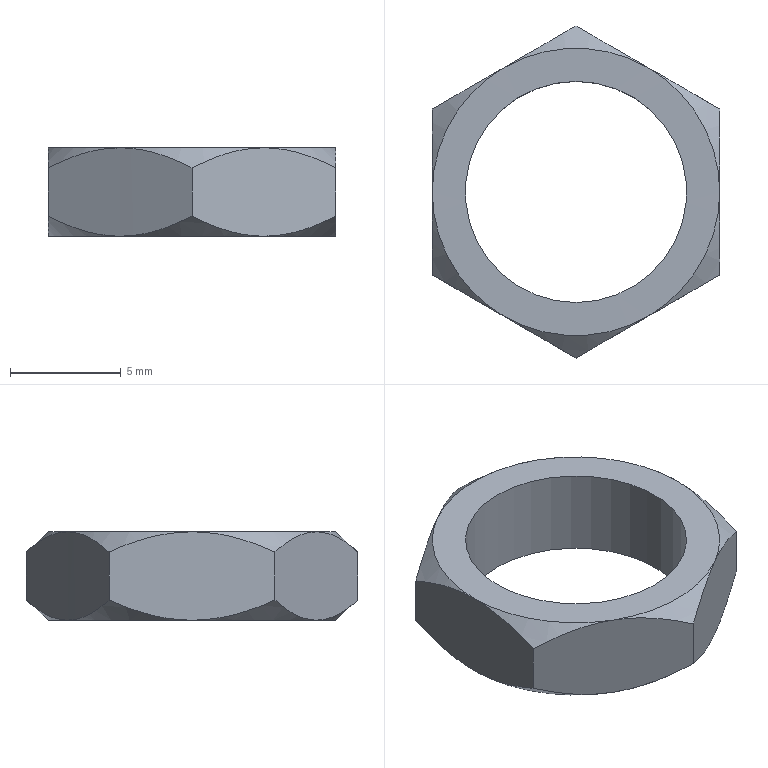Part | STEP file | 1-51.4 | 1 solid | 21 faces | box 13 x 15.011 x 4 mm | volume 263.292 mm3 | cone 12 | plane 8 | cylinder 1 | commonest cylinder face diameters 10 x1